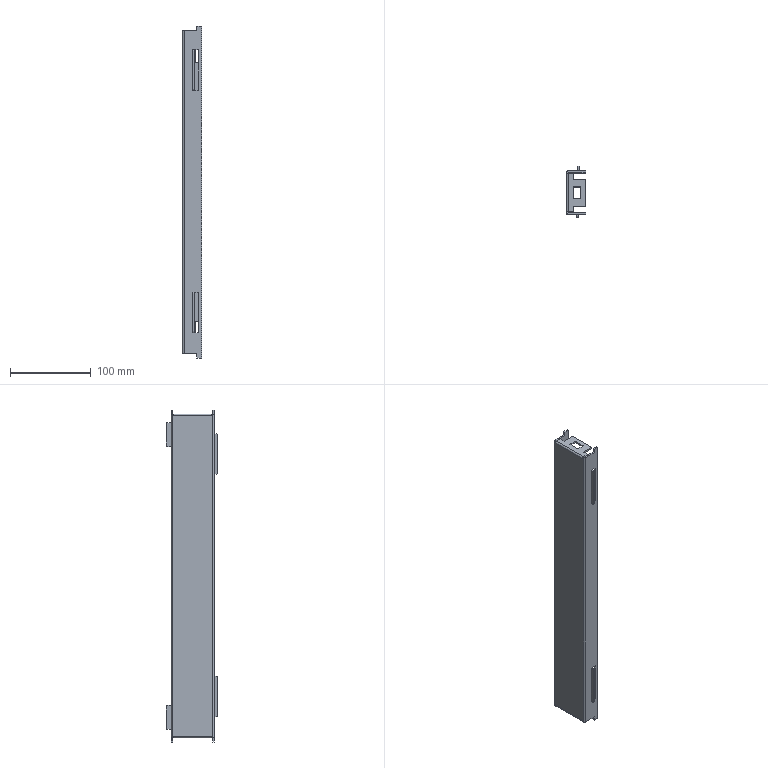Part | NX | features solid 2 | 1 solid | 126 faces | box 23.7 x 63.5 x 411.3 mm | volume 78967 mm3 | plane 110 | cylinder 16 | commonest cylinder face diameters 4 x16